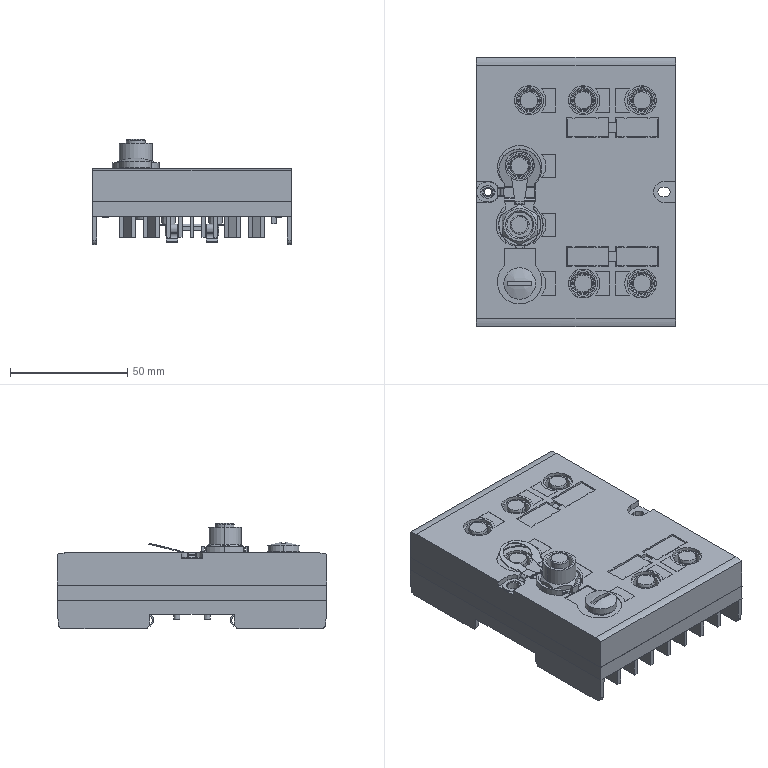Part | STEP file | 1 solid | 954 faces | box 85 x 115 x 44.75 mm | volume 205156 mm3 | plane 567 | cylinder 266 | cone 72 | spline 33 | other 16 | commonest cylinder face diameters 0.56 x32 0.984 x28 1.5 x14 4.2 x14 7.85 x14 9.8 x14